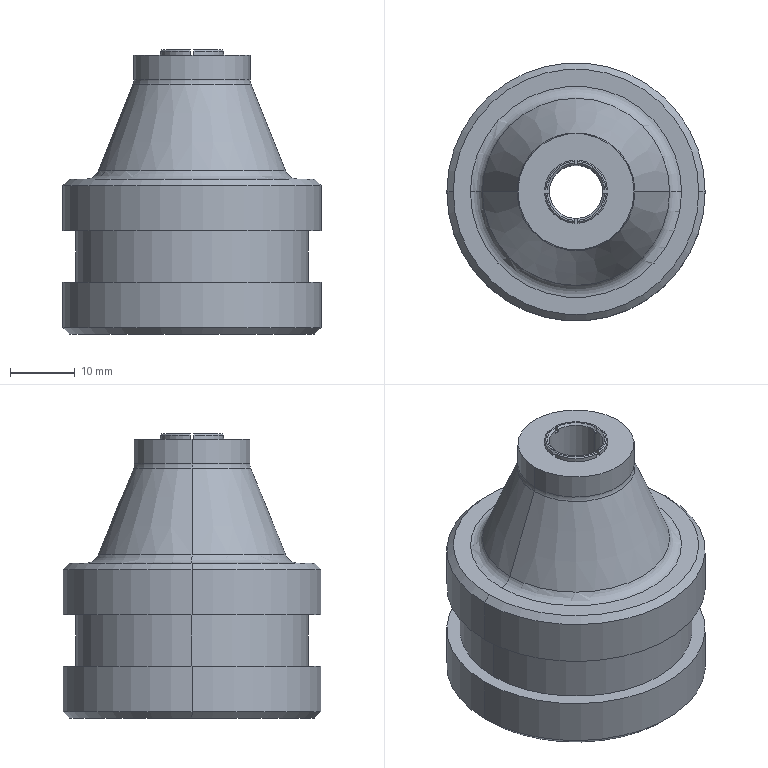Part | STEP file | 001-009-Riveting mechanism upper die insert | 1 solid | 49 faces | box 40 x 40 x 44 mm | volume 33830 mm3 | plane 17 | cone 14 | cylinder 14 | torus 4 | commonest cylinder face diameters 9.8 x4 40 x4 8.3 x2 18 x2 36 x2